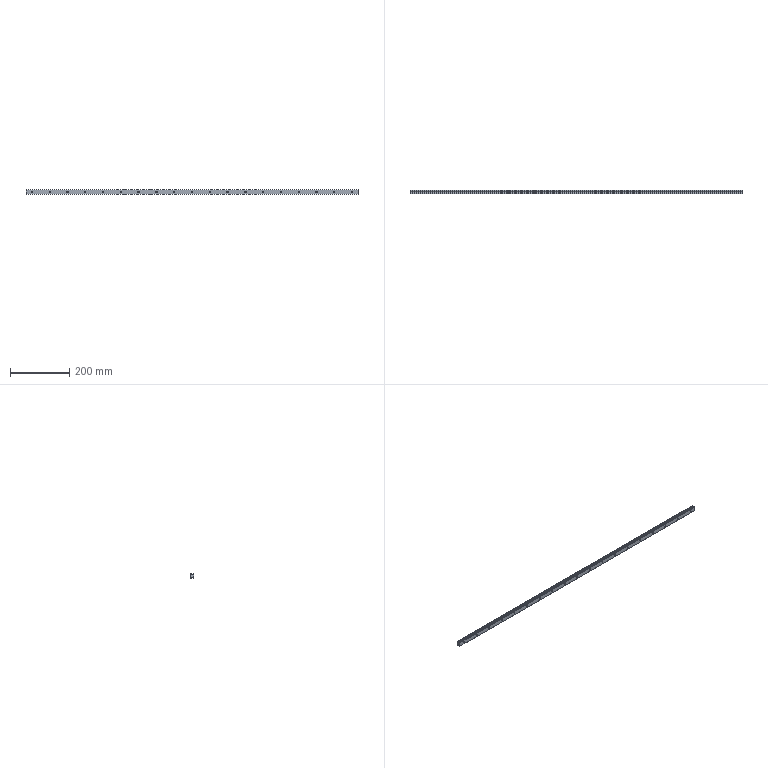Part | NX | 1 solid | 101 faces | box 1120 x 13 x 15 mm | volume 180901 mm3 | cylinder 60 | plane 41 | commonest cylinder face diameters 4.5 x19 7.5 x19 0.6 x6 2.861 x4 0.398 x2 0.545 x2